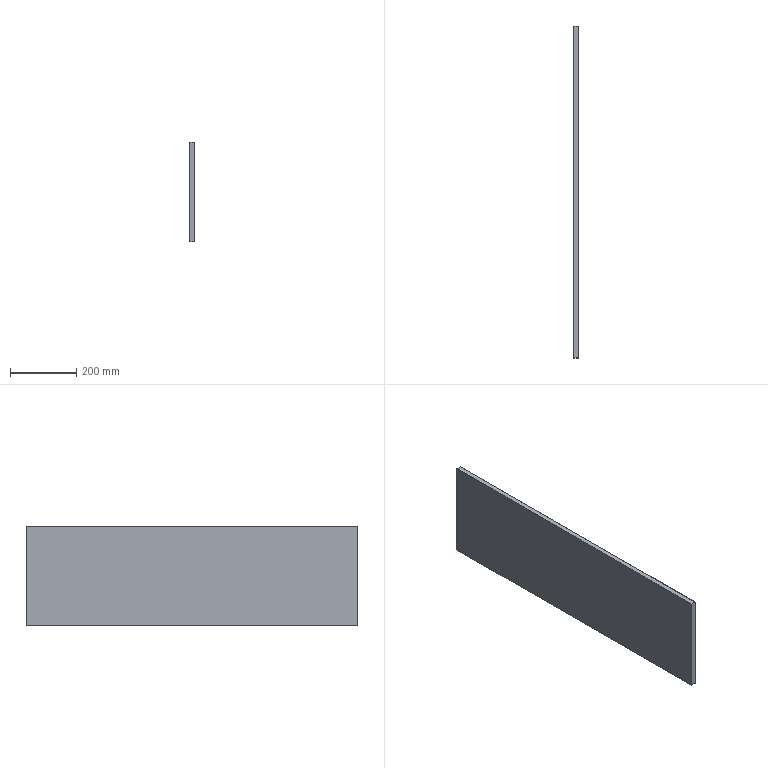Part | STEP file | HJDX-200 | 1 solid | 26 faces | box 16 x 1000 x 300 mm | volume 4799343 mm3 | plane 26
STEP:
#1=CARTESIAN_POINT('',(16.,-499.5,-149.5));
#2=VERTEX_POINT('',#1);
#3=CARTESIAN_POINT('',(16.,-499.5,149.5));
#4=VERTEX_POINT('',#3);
#5=CARTESIAN_POINT('',(16.,-499.5,0.));
#6=DIRECTION('',(0.,0.,1.));
#7=VECTOR('',#6,1000.);
#8=LINE('',#5,#7);
#9=EDGE_CURVE('',#2,#4,#8,.T.);
#10=ORIENTED_EDGE('',*,*,#9,.F.);
#11=CARTESIAN_POINT('',(16.,499.5,-149.5));
#12=VERTEX_POINT('',#11);
#13=CARTESIAN_POINT('',(16.,0.,-149.5));
#14=DIRECTION('',(0.,-1.,0.));
#15=VECTOR('',#14,1000.);
#16=LINE('',#13,#15);
#17=EDGE_CURVE('',#12,#2,#16,.T.);
#18=ORIENTED_EDGE('',*,*,#17,.F.);
#19=CARTESIAN_POINT('',(16.,499.5,149.5));
#20=VERTEX_POINT('',#19);
#21=CARTESIAN_POINT('',(16.,499.5,0.));
#22=DIRECTION('',(0.,0.,-1.));
#23=VECTOR('',#22,1000.);
#24=LINE('',#21,#23);
#25=EDGE_CURVE('',#20,#12,#24,.T.);
#26=ORIENTED_EDGE('',*,*,#25,.F.);
#27=CARTESIAN_POINT('',(16.,0.,149.5));
#28=DIRECTION('',(0.,1.,0.));
#29=VECTOR('',#28,1000.);
#30=LINE('',#27,#29);
#31=EDGE_CURVE('',#4,#20,#30,.T.);
#32=ORIENTED_EDGE('',*,*,#31,.F.);
#33=EDGE_LOOP('',(#10,#18,#26,#32));
#34=FACE_OUTER_BOUND('',#33,.T.);
#35=CARTESIAN_POINT('',(16.,0.,0.));
#36=DIRECTION('',(-1.,0.,0.));
#37=DIRECTION('',(0.,0.,1.));
#38=AXIS2_PLACEMENT_3D('',#35,#36,#37);
#39=PLANE('',#38);
#40=ADVANCED_FACE('',(#34),#39,.F.);
#41=CARTESIAN_POINT('',(15.5,-499.5,150.));
#42=VERTEX_POINT('',#41);
#43=CARTESIAN_POINT('',(15.5,499.5,150.));
#44=VERTEX_POINT('',#43);
#45=CARTESIAN_POINT('',(15.5,0.,150.));
#46=DIRECTION('',(0.,1.,0.));
#47=VECTOR('',#46,1000.);
#48=LINE('',#45,#47);
#49=EDGE_CURVE('',#42,#44,#48,.T.);
#50=ORIENTED_EDGE('',*,*,#49,.F.);
#51=CARTESIAN_POINT('',(16.,-499.5,149.5));
#52=DIRECTION('',(-0.7071,0.,0.7071));
#53=VECTOR('',#52,1000.);
#54=LINE('',#51,#53);
#55=EDGE_CURVE('',#4,#42,#54,.T.);
#56=ORIENTED_EDGE('',*,*,#55,.F.);
#57=ORIENTED_EDGE('',*,*,#31,.T.);
#58=CARTESIAN_POINT('',(16.,499.5,149.5));
#59=DIRECTION('',(0.7071,0.,-0.7071));
#60=VECTOR('',#59,1000.);
#61=LINE('',#58,#60);
#62=EDGE_CURVE('',#44,#20,#61,.T.);
#63=ORIENTED_EDGE('',*,*,#62,.F.);
#64=EDGE_LOOP('',(#50,#56,#57,#63));
#65=FACE_OUTER_BOUND('',#64,.T.);
#66=CARTESIAN_POINT('',(16.,0.,149.5));
#67=DIRECTION('',(-0.7071,0.,-0.7071));
#68=DIRECTION('',(-0.7071,0.,0.7071));
#69=AXIS2_PLACEMENT_3D('',#66,#67,#68);
#70=PLANE('',#69);
#71=ADVANCED_FACE('',(#65),#70,.F.);
#72=CARTESIAN_POINT('',(15.5,-500.,-149.5));
#73=VERTEX_POINT('',#72);
#74=CARTESIAN_POINT('',(15.5,-500.,149.5));
#75=VERTEX_POINT('',#74);
#76=CARTESIAN_POINT('',(15.5,-500.,0.));
#77=DIRECTION('',(0.,0.,1.));
#78=VECTOR('',#77,1000.);
#79=LINE('',#76,#78);
#80=EDGE_CURVE('',#73,#75,#79,.T.);
#81=ORIENTED_EDGE('',*,*,#80,.F.);
#82=CARTESIAN_POINT('',(16.,-499.5,-149.5));
#83=DIRECTION('',(-0.7071,-0.7071,0.));
#84=VECTOR('',#83,1000.);
#85=LINE('',#82,#84);
#86=EDGE_CURVE('',#2,#73,#85,.T.);
#87=ORIENTED_EDGE('',*,*,#86,.F.);
#88=ORIENTED_EDGE('',*,*,#9,.T.);
#89=CARTESIAN_POINT('',(16.,-499.5,149.5));
#90=DIRECTION('',(0.7071,0.7071,0.));
#91=VECTOR('',#90,1000.);
#92=LINE('',#89,#91);
#93=EDGE_CURVE('',#75,#4,#92,.T.);
#94=ORIENTED_EDGE('',*,*,#93,.F.);
#95=EDGE_LOOP('',(#81,#87,#88,#94));
#96=FACE_OUTER_BOUND('',#95,.T.);
#97=CARTESIAN_POINT('',(16.,-499.5,0.));
#98=DIRECTION('',(-0.7071,0.7071,0.));
#99=DIRECTION('',(-0.7071,-0.7071,0.));
#100=AXIS2_PLACEMENT_3D('',#97,#98,#99);
#101=PLANE('',#100);
#102=ADVANCED_FACE('',(#96),#101,.F.);
#103=ORIENTED_EDGE('',*,*,#17,.T.);
#104=CARTESIAN_POINT('',(15.5,-499.5,-150.));
#105=VERTEX_POINT('',#104);
#106=CARTESIAN_POINT('',(16.,-499.5,-149.5));
#107=DIRECTION('',(0.7071,0.,0.7071));
#108=VECTOR('',#107,1000.);
#109=LINE('',#106,#108);
#110=EDGE_CURVE('',#105,#2,#109,.T.);
#111=ORIENTED_EDGE('',*,*,#110,.F.);
#112=CARTESIAN_POINT('',(15.5,499.5,-150.));
#113=VERTEX_POINT('',#112);
#114=CARTESIAN_POINT('',(15.5,0.,-150.));
#115=DIRECTION('',(0.,-1.,0.));
#116=VECTOR('',#115,1000.);
#117=LINE('',#114,#116);
#118=EDGE_CURVE('',#113,#105,#117,.T.);
#119=ORIENTED_EDGE('',*,*,#118,.F.);
#120=CARTESIAN_POINT('',(16.,499.5,-149.5));
#121=DIRECTION('',(-0.7071,0.,-0.7071));
#122=VECTOR('',#121,1000.);
#123=LINE('',#120,#122);
#124=EDGE_CURVE('',#12,#113,#123,.T.);
#125=ORIENTED_EDGE('',*,*,#124,.F.);
#126=EDGE_LOOP('',(#103,#111,#119,#125));
#127=FACE_OUTER_BOUND('',#126,.T.);
#128=CARTESIAN_POINT('',(16.,0.,-149.5));
#129=DIRECTION('',(-0.7071,0.,0.7071));
#130=DIRECTION('',(0.7071,0.,0.7071));
#131=AXIS2_PLACEMENT_3D('',#128,#129,#130);
#132=PLANE('',#131);
#133=ADVANCED_FACE('',(#127),#132,.F.);
#134=ORIENTED_EDGE('',*,*,#25,.T.);
#135=CARTESIAN_POINT('',(15.5,500.,-149.5));
#136=VERTEX_POINT('',#135);
#137=CARTESIAN_POINT('',(16.,499.5,-149.5));
#138=DIRECTION('',(0.7071,-0.7071,0.));
#139=VECTOR('',#138,1000.);
#140=LINE('',#137,#139);
#141=EDGE_CURVE('',#136,#12,#140,.T.);
#142=ORIENTED_EDGE('',*,*,#141,.F.);
#143=CARTESIAN_POINT('',(15.5,500.,149.5));
#144=VERTEX_POINT('',#143);
#145=CARTESIAN_POINT('',(15.5,500.,0.));
#146=DIRECTION('',(0.,0.,-1.));
#147=VECTOR('',#146,1000.);
#148=LINE('',#145,#147);
#149=EDGE_CURVE('',#144,#136,#148,.T.);
#150=ORIENTED_EDGE('',*,*,#149,.F.);
#151=CARTESIAN_POINT('',(16.,499.5,149.5));
#152=DIRECTION('',(-0.7071,0.7071,0.));
#153=VECTOR('',#152,1000.);
#154=LINE('',#151,#153);
#155=EDGE_CURVE('',#20,#144,#154,.T.);
#156=ORIENTED_EDGE('',*,*,#155,.F.);
#157=EDGE_LOOP('',(#134,#142,#150,#156));
#158=FACE_OUTER_BOUND('',#157,.T.);
#159=CARTESIAN_POINT('',(16.,499.5,0.));
#160=DIRECTION('',(-0.7071,-0.7071,0.));
#161=DIRECTION('',(0.7071,-0.7071,0.));
#162=AXIS2_PLACEMENT_3D('',#159,#160,#161);
#163=PLANE('',#162);
#164=ADVANCED_FACE('',(#158),#163,.F.);
#165=CARTESIAN_POINT('',(15.5,499.5,150.));
#166=DIRECTION('',(0.,-0.7071,0.7071));
#167=VECTOR('',#166,1000.);
#168=LINE('',#165,#167);
#169=EDGE_CURVE('',#144,#44,#168,.T.);
#170=ORIENTED_EDGE('',*,*,#169,.T.);
#171=ORIENTED_EDGE('',*,*,#62,.T.);
#172=ORIENTED_EDGE('',*,*,#155,.T.);
#173=EDGE_LOOP('',(#170,#171,#172));
#174=FACE_OUTER_BOUND('',#173,.T.);
#175=CARTESIAN_POINT('',(15.5,500.,149.5));
#176=DIRECTION('',(0.5774,0.5774,0.5774));
#177=DIRECTION('',(0.7071,0.,-0.7071));
#178=AXIS2_PLACEMENT_3D('',#175,#176,#177);
#179=PLANE('',#178);
#180=ADVANCED_FACE('',(#174),#179,.T.);
#181=CARTESIAN_POINT('',(0.5,499.5,150.));
#182=VERTEX_POINT('',#181);
#183=CARTESIAN_POINT('',(16.,499.5,150.));
#184=DIRECTION('',(1.,0.,0.));
#185=VECTOR('',#184,1000.);
#186=LINE('',#183,#185);
#187=EDGE_CURVE('',#182,#44,#186,.T.);
#188=ORIENTED_EDGE('',*,*,#187,.F.);
#189=CARTESIAN_POINT('',(0.5,-499.5,150.));
#190=VERTEX_POINT('',#189);
#191=CARTESIAN_POINT('',(0.5,-500.,150.));
#192=DIRECTION('',(0.,1.,0.));
#193=VECTOR('',#192,1000.);
#194=LINE('',#191,#193);
#195=EDGE_CURVE('',#190,#182,#194,.T.);
#196=ORIENTED_EDGE('',*,*,#195,.F.);
#197=CARTESIAN_POINT('',(16.,-499.5,150.));
#198=DIRECTION('',(-1.,0.,0.));
#199=VECTOR('',#198,1000.);
#200=LINE('',#197,#199);
#201=EDGE_CURVE('',#42,#190,#200,.T.);
#202=ORIENTED_EDGE('',*,*,#201,.F.);
#203=ORIENTED_EDGE('',*,*,#49,.T.);
#204=EDGE_LOOP('',(#188,#196,#202,#203));
#205=FACE_OUTER_BOUND('',#204,.T.);
#206=CARTESIAN_POINT('',(16.,-500.,150.));
#207=DIRECTION('',(0.,0.,-1.));
#208=DIRECTION('',(-1.,0.,0.));
#209=AXIS2_PLACEMENT_3D('',#206,#207,#208);
#210=PLANE('',#209);
#211=ADVANCED_FACE('',(#205),#210,.F.);
#212=CARTESIAN_POINT('',(15.5,-499.5,150.));
#213=DIRECTION('',(0.,-0.7071,-0.7071));
#214=VECTOR('',#213,1000.);
#215=LINE('',#212,#214);
#216=EDGE_CURVE('',#42,#75,#215,.T.);
#217=ORIENTED_EDGE('',*,*,#216,.T.);
#218=ORIENTED_EDGE('',*,*,#93,.T.);
#219=ORIENTED_EDGE('',*,*,#55,.T.);
#220=EDGE_LOOP('',(#217,#218,#219));
#221=FACE_OUTER_BOUND('',#220,.T.);
#222=CARTESIAN_POINT('',(15.5,-499.5,150.));
#223=DIRECTION('',(0.5774,-0.5774,0.5774));
#224=DIRECTION('',(0.7071,0.,-0.7071));
#225=AXIS2_PLACEMENT_3D('',#222,#223,#224);
#226=PLANE('',#225);
#227=ADVANCED_FACE('',(#221),#226,.T.);
#228=CARTESIAN_POINT('',(0.5,-500.,-149.5));
#229=VERTEX_POINT('',#228);
#230=CARTESIAN_POINT('',(16.,-500.,-149.5));
#231=DIRECTION('',(-1.,0.,0.));
#232=VECTOR('',#231,1000.);
#233=LINE('',#230,#232);
#234=EDGE_CURVE('',#73,#229,#233,.T.);
#235=ORIENTED_EDGE('',*,*,#234,.F.);
#236=ORIENTED_EDGE('',*,*,#80,.T.);
#237=CARTESIAN_POINT('',(0.5,-500.,149.5));
#238=VERTEX_POINT('',#237);
#239=CARTESIAN_POINT('',(16.,-500.,149.5));
#240=DIRECTION('',(1.,0.,0.));
#241=VECTOR('',#240,1000.);
#242=LINE('',#239,#241);
#243=EDGE_CURVE('',#238,#75,#242,.T.);
#244=ORIENTED_EDGE('',*,*,#243,.F.);
#245=CARTESIAN_POINT('',(0.5,-500.,150.));
#246=DIRECTION('',(0.,0.,1.));
#247=VECTOR('',#246,1000.);
#248=LINE('',#245,#247);
#249=EDGE_CURVE('',#229,#238,#248,.T.);
#250=ORIENTED_EDGE('',*,*,#249,.F.);
#251=EDGE_LOOP('',(#235,#236,#244,#250));
#252=FACE_OUTER_BOUND('',#251,.T.);
#253=CARTESIAN_POINT('',(16.,-500.,150.));
#254=DIRECTION('',(0.,1.,0.));
#255=DIRECTION('',(0.,0.,1.));
#256=AXIS2_PLACEMENT_3D('',#253,#254,#255);
#257=PLANE('',#256);
#258=ADVANCED_FACE('',(#252),#257,.F.);
#259=ORIENTED_EDGE('',*,*,#86,.T.);
#260=CARTESIAN_POINT('',(15.5,-500.,-149.5));
#261=DIRECTION('',(0.,0.7071,-0.7071));
#262=VECTOR('',#261,1000.);
#263=LINE('',#260,#262);
#264=EDGE_CURVE('',#73,#105,#263,.T.);
#265=ORIENTED_EDGE('',*,*,#264,.T.);
#266=ORIENTED_EDGE('',*,*,#110,.T.);
#267=EDGE_LOOP('',(#259,#265,#266));
#268=FACE_OUTER_BOUND('',#267,.T.);
#269=CARTESIAN_POINT('',(15.5,-500.,-149.5));
#270=DIRECTION('',(0.5774,-0.5774,-0.5774));
#271=DIRECTION('',(-0.7071,0.,-0.7071));
#272=AXIS2_PLACEMENT_3D('',#269,#270,#271);
#273=PLANE('',#272);
#274=ADVANCED_FACE('',(#268),#273,.T.);
#275=ORIENTED_EDGE('',*,*,#141,.T.);
#276=ORIENTED_EDGE('',*,*,#124,.T.);
#277=CARTESIAN_POINT('',(15.5,500.,-149.5));
#278=DIRECTION('',(0.,0.7071,0.7071));
#279=VECTOR('',#278,1000.);
#280=LINE('',#277,#279);
#281=EDGE_CURVE('',#113,#136,#280,.T.);
#282=ORIENTED_EDGE('',*,*,#281,.T.);
#283=EDGE_LOOP('',(#275,#276,#282));
#284=FACE_OUTER_BOUND('',#283,.T.);
#285=CARTESIAN_POINT('',(15.5,499.5,-150.));
#286=DIRECTION('',(0.5774,0.5774,-0.5774));
#287=DIRECTION('',(-0.7071,0.,-0.7071));
#288=AXIS2_PLACEMENT_3D('',#285,#286,#287);
#289=PLANE('',#288);
#290=ADVANCED_FACE('',(#284),#289,.T.);
#291=CARTESIAN_POINT('',(0.5,499.5,-150.));
#292=VERTEX_POINT('',#291);
#293=CARTESIAN_POINT('',(0.5,-499.5,-150.));
#294=VERTEX_POINT('',#293);
#295=CARTESIAN_POINT('',(0.5,-500.,-150.));
#296=DIRECTION('',(0.,-1.,0.));
#297=VECTOR('',#296,1000.);
#298=LINE('',#295,#297);
#299=EDGE_CURVE('',#292,#294,#298,.T.);
#300=ORIENTED_EDGE('',*,*,#299,.F.);
#301=CARTESIAN_POINT('',(16.,499.5,-150.));
#302=DIRECTION('',(-1.,0.,0.));
#303=VECTOR('',#302,1000.);
#304=LINE('',#301,#303);
#305=EDGE_CURVE('',#113,#292,#304,.T.);
#306=ORIENTED_EDGE('',*,*,#305,.F.);
#307=ORIENTED_EDGE('',*,*,#118,.T.);
#308=CARTESIAN_POINT('',(16.,-499.5,-150.));
#309=DIRECTION('',(1.,0.,0.));
#310=VECTOR('',#309,1000.);
#311=LINE('',#308,#310);
#312=EDGE_CURVE('',#294,#105,#311,.T.);
#313=ORIENTED_EDGE('',*,*,#312,.F.);
#314=EDGE_LOOP('',(#300,#306,#307,#313));
#315=FACE_OUTER_BOUND('',#314,.T.);
#316=CARTESIAN_POINT('',(16.,-500.,-150.));
#317=DIRECTION('',(0.,0.,1.));
#318=DIRECTION('',(1.,0.,0.));
#319=AXIS2_PLACEMENT_3D('',#316,#317,#318);
#320=PLANE('',#319);
#321=ADVANCED_FACE('',(#315),#320,.F.);
#322=CARTESIAN_POINT('',(0.5,500.,149.5));
#323=VERTEX_POINT('',#322);
#324=CARTESIAN_POINT('',(0.5,500.,-149.5));
#325=VERTEX_POINT('',#324);
#326=CARTESIAN_POINT('',(0.5,500.,150.));
#327=DIRECTION('',(0.,0.,-1.));
#328=VECTOR('',#327,1000.);
#329=LINE('',#326,#328);
#330=EDGE_CURVE('',#323,#325,#329,.T.);
#331=ORIENTED_EDGE('',*,*,#330,.F.);
#332=CARTESIAN_POINT('',(16.,500.,149.5));
#333=DIRECTION('',(-1.,0.,0.));
#334=VECTOR('',#333,1000.);
#335=LINE('',#332,#334);
#336=EDGE_CURVE('',#144,#323,#335,.T.);
#337=ORIENTED_EDGE('',*,*,#336,.F.);
#338=ORIENTED_EDGE('',*,*,#149,.T.);
#339=CARTESIAN_POINT('',(16.,500.,-149.5));
#340=DIRECTION('',(1.,0.,0.));
#341=VECTOR('',#340,1000.);
#342=LINE('',#339,#341);
#343=EDGE_CURVE('',#325,#136,#342,.T.);
#344=ORIENTED_EDGE('',*,*,#343,.F.);
#345=EDGE_LOOP('',(#331,#337,#338,#344));
#346=FACE_OUTER_BOUND('',#345,.T.);
#347=CARTESIAN_POINT('',(16.,500.,150.));
#348=DIRECTION('',(0.,-1.,0.));
#349=DIRECTION('',(0.,0.,-1.));
#350=AXIS2_PLACEMENT_3D('',#347,#348,#349);
#351=PLANE('',#350);
#352=ADVANCED_FACE('',(#346),#351,.F.);
#353=ORIENTED_EDGE('',*,*,#336,.T.);
#354=CARTESIAN_POINT('',(0.5,499.5,150.));
#355=DIRECTION('',(0.,0.7071,-0.7071));
#356=VECTOR('',#355,1000.);
#357=LINE('',#354,#356);
#358=EDGE_CURVE('',#182,#323,#357,.T.);
#359=ORIENTED_EDGE('',*,*,#358,.F.);
#360=ORIENTED_EDGE('',*,*,#187,.T.);
#361=ORIENTED_EDGE('',*,*,#169,.F.);
#362=EDGE_LOOP('',(#353,#359,#360,#361));
#363=FACE_OUTER_BOUND('',#362,.T.);
#364=CARTESIAN_POINT('',(16.,499.5,150.));
#365=DIRECTION('',(0.,-0.7071,-0.7071));
#366=DIRECTION('',(0.,0.7071,-0.7071));
#367=AXIS2_PLACEMENT_3D('',#364,#365,#366);
#368=PLANE('',#367);
#369=ADVANCED_FACE('',(#363),#368,.F.);
#370=CARTESIAN_POINT('',(0.,-499.5,149.5));
#371=VERTEX_POINT('',#370);
#372=CARTESIAN_POINT('',(0.5,-499.5,150.));
#373=DIRECTION('',(0.7071,0.,0.7071));
#374=VECTOR('',#373,1000.);
#375=LINE('',#372,#374);
#376=EDGE_CURVE('',#371,#190,#375,.T.);
#377=ORIENTED_EDGE('',*,*,#376,.T.);
#378=ORIENTED_EDGE('',*,*,#195,.T.);
#379=CARTESIAN_POINT('',(0.,499.5,149.5));
#380=VERTEX_POINT('',#379);
#381=CARTESIAN_POINT('',(0.5,499.5,150.));
#382=DIRECTION('',(-0.7071,0.,-0.7071));
#383=VECTOR('',#382,1000.);
#384=LINE('',#381,#383);
#385=EDGE_CURVE('',#182,#380,#384,.T.);
#386=ORIENTED_EDGE('',*,*,#385,.T.);
#387=CARTESIAN_POINT('',(0.,-500.,149.5));
#388=DIRECTION('',(0.,-1.,0.));
#389=VECTOR('',#388,1000.);
#390=LINE('',#387,#389);
#391=EDGE_CURVE('',#380,#371,#390,.T.);
#392=ORIENTED_EDGE('',*,*,#391,.T.);
#393=EDGE_LOOP('',(#377,#378,#386,#392));
#394=FACE_OUTER_BOUND('',#393,.T.);
#395=CARTESIAN_POINT('',(0.5,-500.,150.));
#396=DIRECTION('',(-0.7071,0.,0.7071));
#397=DIRECTION('',(0.7071,0.,0.7071));
#398=AXIS2_PLACEMENT_3D('',#395,#396,#397);
#399=PLANE('',#398);
#400=ADVANCED_FACE('',(#394),#399,.T.);
#401=ORIENTED_EDGE('',*,*,#201,.T.);
#402=CARTESIAN_POINT('',(0.5,-500.,149.5));
#403=DIRECTION('',(0.,0.7071,0.7071));
#404=VECTOR('',#403,1000.);
#405=LINE('',#402,#404);
#406=EDGE_CURVE('',#238,#190,#405,.T.);
#407=ORIENTED_EDGE('',*,*,#406,.F.);
#408=ORIENTED_EDGE('',*,*,#243,.T.);
#409=ORIENTED_EDGE('',*,*,#216,.F.);
#410=EDGE_LOOP('',(#401,#407,#408,#409));
#411=FACE_OUTER_BOUND('',#410,.T.);
#412=CARTESIAN_POINT('',(16.,-500.,149.5));
#413=DIRECTION('',(0.,0.7071,-0.7071));
#414=DIRECTION('',(0.,0.7071,0.7071));
#415=AXIS2_PLACEMENT_3D('',#412,#413,#414);
#416=PLANE('',#415);
#417=ADVANCED_FACE('',(#411),#416,.F.);
#418=CARTESIAN_POINT('',(0.,-499.5,-149.5));
#419=VERTEX_POINT('',#418);
#420=CARTESIAN_POINT('',(0.5,-500.,-149.5));
#421=DIRECTION('',(0.7071,-0.7071,0.));
#422=VECTOR('',#421,1000.);
#423=LINE('',#420,#422);
#424=EDGE_CURVE('',#419,#229,#423,.T.);
#425=ORIENTED_EDGE('',*,*,#424,.T.);
#426=ORIENTED_EDGE('',*,*,#249,.T.);
#427=CARTESIAN_POINT('',(0.5,-500.,149.5));
#428=DIRECTION('',(-0.7071,0.7071,0.));
#429=VECTOR('',#428,1000.);
#430=LINE('',#427,#429);
#431=EDGE_CURVE('',#238,#371,#430,.T.);
#432=ORIENTED_EDGE('',*,*,#431,.T.);
#433=CARTESIAN_POINT('',(0.,-499.5,150.));
#434=DIRECTION('',(0.,0.,-1.));
#435=VECTOR('',#434,1000.);
#436=LINE('',#433,#435);
#437=EDGE_CURVE('',#371,#419,#436,.T.);
#438=ORIENTED_EDGE('',*,*,#437,.T.);
#439=EDGE_LOOP('',(#425,#426,#432,#438));
#440=FACE_OUTER_BOUND('',#439,.T.);
#441=CARTESIAN_POINT('',(0.5,-500.,150.));
#442=DIRECTION('',(-0.7071,-0.7071,0.));
#443=DIRECTION('',(0.7071,-0.7071,0.));
#444=AXIS2_PLACEMENT_3D('',#441,#442,#443);
#445=PLANE('',#444);
#446=ADVANCED_FACE('',(#440),#445,.T.);
#447=ORIENTED_EDGE('',*,*,#234,.T.);
#448=CARTESIAN_POINT('',(0.5,-499.5,-150.));
#449=DIRECTION('',(0.,-0.7071,0.7071));
#450=VECTOR('',#449,1000.);
#451=LINE('',#448,#450);
#452=EDGE_CURVE('',#294,#229,#451,.T.);
#453=ORIENTED_EDGE('',*,*,#452,.F.);
#454=ORIENTED_EDGE('',*,*,#312,.T.);
#455=ORIENTED_EDGE('',*,*,#264,.F.);
#456=EDGE_LOOP('',(#447,#453,#454,#455));
#457=FACE_OUTER_BOUND('',#456,.T.);
#458=CARTESIAN_POINT('',(16.,-499.5,-150.));
#459=DIRECTION('',(0.,0.7071,0.7071));
#460=DIRECTION('',(0.,-0.7071,0.7071));
#461=AXIS2_PLACEMENT_3D('',#458,#459,#460);
#462=PLANE('',#461);
#463=ADVANCED_FACE('',(#457),#462,.F.);
#464=CARTESIAN_POINT('',(0.5,-499.5,-150.));
#465=DIRECTION('',(-0.7071,0.,0.7071));
#466=VECTOR('',#465,1000.);
#467=LINE('',#464,#466);
#468=EDGE_CURVE('',#294,#419,#467,.T.);
#469=ORIENTED_EDGE('',*,*,#468,.T.);
#470=CARTESIAN_POINT('',(0.,499.5,-149.5));
#471=VERTEX_POINT('',#470);
#472=CARTESIAN_POINT('',(0.,-500.,-149.5));
#473=DIRECTION('',(0.,1.,0.));
#474=VECTOR('',#473,1000.);
#475=LINE('',#472,#474);
#476=EDGE_CURVE('',#419,#471,#475,.T.);
#477=ORIENTED_EDGE('',*,*,#476,.T.);
#478=CARTESIAN_POINT('',(0.5,499.5,-150.));
#479=DIRECTION('',(0.7071,0.,-0.7071));
#480=VECTOR('',#479,1000.);
#481=LINE('',#478,#480);
#482=EDGE_CURVE('',#471,#292,#481,.T.);
#483=ORIENTED_EDGE('',*,*,#482,.T.);
#484=ORIENTED_EDGE('',*,*,#299,.T.);
#485=EDGE_LOOP('',(#469,#477,#483,#484));
#486=FACE_OUTER_BOUND('',#485,.T.);
#487=CARTESIAN_POINT('',(0.5,-500.,-150.));
#488=DIRECTION('',(-0.7071,0.,-0.7071));
#489=DIRECTION('',(-0.7071,0.,0.7071));
#490=AXIS2_PLACEMENT_3D('',#487,#488,#489);
#491=PLANE('',#490);
#492=ADVANCED_FACE('',(#486),#491,.T.);
#493=ORIENTED_EDGE('',*,*,#343,.T.);
#494=ORIENTED_EDGE('',*,*,#281,.F.);
#495=ORIENTED_EDGE('',*,*,#305,.T.);
#496=CARTESIAN_POINT('',(0.5,500.,-149.5));
#497=DIRECTION('',(0.,-0.7071,-0.7071));
#498=VECTOR('',#497,1000.);
#499=LINE('',#496,#498);
#500=EDGE_CURVE('',#325,#292,#499,.T.);
#501=ORIENTED_EDGE('',*,*,#500,.F.);
#502=EDGE_LOOP('',(#493,#494,#495,#501));
#503=FACE_OUTER_BOUND('',#502,.T.);
#504=CARTESIAN_POINT('',(16.,500.,-149.5));
#505=DIRECTION('',(0.,-0.7071,0.7071));
#506=DIRECTION('',(0.,-0.7071,-0.7071));
#507=AXIS2_PLACEMENT_3D('',#504,#505,#506);
#508=PLANE('',#507);
#509=ADVANCED_FACE('',(#503),#508,.F.);
#510=CARTESIAN_POINT('',(0.5,500.,-149.5));
#511=DIRECTION('',(-0.7071,-0.7071,0.));
#512=VECTOR('',#511,1000.);
#513=LINE('',#510,#512);
#514=EDGE_CURVE('',#325,#471,#513,.T.);
#515=ORIENTED_EDGE('',*,*,#514,.T.);
#516=CARTESIAN_POINT('',(0.,499.5,150.));
#517=DIRECTION('',(0.,0.,1.));
#518=VECTOR('',#517,1000.);
#519=LINE('',#516,#518);
#520=EDGE_CURVE('',#471,#380,#519,.T.);
#521=ORIENTED_EDGE('',*,*,#520,.T.);
#522=CARTESIAN_POINT('',(0.5,500.,149.5));
#523=DIRECTION('',(0.7071,0.7071,0.));
#524=VECTOR('',#523,1000.);
#525=LINE('',#522,#524);
#526=EDGE_CURVE('',#380,#323,#525,.T.);
#527=ORIENTED_EDGE('',*,*,#526,.T.);
#528=ORIENTED_EDGE('',*,*,#330,.T.);
#529=EDGE_LOOP('',(#515,#521,#527,#528));
#530=FACE_OUTER_BOUND('',#529,.T.);
#531=CARTESIAN_POINT('',(0.5,500.,150.));
#532=DIRECTION('',(-0.7071,0.7071,0.));
#533=DIRECTION('',(-0.7071,-0.7071,0.));
#534=AXIS2_PLACEMENT_3D('',#531,#532,#533);
#535=PLANE('',#534);
#536=ADVANCED_FACE('',(#530),#535,.T.);
#537=ORIENTED_EDGE('',*,*,#358,.T.);
#538=ORIENTED_EDGE('',*,*,#526,.F.);
#539=ORIENTED_EDGE('',*,*,#385,.F.);
#540=EDGE_LOOP('',(#537,#538,#539));
#541=FACE_OUTER_BOUND('',#540,.T.);
#542=CARTESIAN_POINT('',(0.5,499.5,150.));
#543=DIRECTION('',(-0.5774,0.5774,0.5774));
#544=DIRECTION('',(0.7071,0.,0.7071));
#545=AXIS2_PLACEMENT_3D('',#542,#543,#544);
#546=PLANE('',#545);
#547=ADVANCED_FACE('',(#541),#546,.T.);
#548=ORIENTED_EDGE('',*,*,#376,.F.);
#549=ORIENTED_EDGE('',*,*,#431,.F.);
#550=ORIENTED_EDGE('',*,*,#406,.T.);
#551=EDGE_LOOP('',(#548,#549,#550));
#552=FACE_OUTER_BOUND('',#551,.T.);
#553=CARTESIAN_POINT('',(0.5,-499.5,150.));
#554=DIRECTION('',(-0.5774,-0.5774,0.5774));
#555=DIRECTION('',(0.7071,0.,0.7071));
#556=AXIS2_PLACEMENT_3D('',#553,#554,#555);
#557=PLANE('',#556);
#558=ADVANCED_FACE('',(#552),#557,.T.);
#559=ORIENTED_EDGE('',*,*,#476,.F.);
#560=ORIENTED_EDGE('',*,*,#437,.F.);
#561=ORIENTED_EDGE('',*,*,#391,.F.);
#562=ORIENTED_EDGE('',*,*,#520,.F.);
#563=EDGE_LOOP('',(#559,#560,#561,#562));
#564=FACE_OUTER_BOUND('',#563,.T.);
#565=CARTESIAN_POINT('',(0.,0.,0.));
#566=DIRECTION('',(-1.,0.,0.));
#567=DIRECTION('',(0.,0.,1.));
#568=AXIS2_PLACEMENT_3D('',#565,#566,#567);
#569=PLANE('',#568);
#570=ADVANCED_FACE('',(#564),#569,.T.);
#571=ORIENTED_EDGE('',*,*,#468,.F.);
#572=ORIENTED_EDGE('',*,*,#452,.T.);
#573=ORIENTED_EDGE('',*,*,#424,.F.);
#574=EDGE_LOOP('',(#571,#572,#573));
#575=FACE_OUTER_BOUND('',#574,.T.);
#576=CARTESIAN_POINT('',(0.5,-499.5,-150.));
#577=DIRECTION('',(-0.5774,-0.5774,-0.5774));
#578=DIRECTION('',(-0.7071,0.,0.7071));
#579=AXIS2_PLACEMENT_3D('',#576,#577,#578);
#580=PLANE('',#579);
#581=ADVANCED_FACE('',(#575),#580,.T.);
#582=ORIENTED_EDGE('',*,*,#500,.T.);
#583=ORIENTED_EDGE('',*,*,#482,.F.);
#584=ORIENTED_EDGE('',*,*,#514,.F.);
#585=EDGE_LOOP('',(#582,#583,#584));
#586=FACE_OUTER_BOUND('',#585,.T.);
#587=CARTESIAN_POINT('',(0.5,500.,-149.5));
#588=DIRECTION('',(-0.5774,0.5774,-0.5774));
#589=DIRECTION('',(-0.7071,0.,0.7071));
#590=AXIS2_PLACEMENT_3D('',#587,#588,#589);
#591=PLANE('',#590);
#592=ADVANCED_FACE('',(#586),#591,.T.);
#593=CLOSED_SHELL('',(#40,#71,#102,#133,#164,#180,#211,#227,#258,#274,#290,#321,#352,#369,#400,#417,#446,#463,#492,#509,#536,#547,#558,#570,#581,#592));
#594=MANIFOLD_SOLID_BREP('',#593);
#595=CARTESIAN_POINT('',(0.,0.,0.));
#596=DIRECTION('',(0.,0.,1.));
#597=DIRECTION('',(1.,0.,0.));
#598=AXIS2_PLACEMENT_3D('',#595,#596,#597);
#599=(LENGTH_UNIT()NAMED_UNIT(*)SI_UNIT(.MILLI.,.METRE.));
#600=UNCERTAINTY_MEASURE_WITH_UNIT(LENGTH_MEASURE(0.00001),#599,'','');
#601=(NAMED_UNIT(*)PLANE_ANGLE_UNIT()SI_UNIT($,.RADIAN.));
#602=(NAMED_UNIT(*)SI_UNIT($,.STERADIAN.)SOLID_ANGLE_UNIT());
#603=(GEOMETRIC_REPRESENTATION_CONTEXT(3)GLOBAL_UNCERTAINTY_ASSIGNED_CONTEXT((#600))GLOBAL_UNIT_ASSIGNED_CONTEXT((#599,#601,#602))REPRESENTATION_CONTEXT('',''));
#604=ADVANCED_BREP_SHAPE_REPRESENTATION('',(#594,#598),#603);